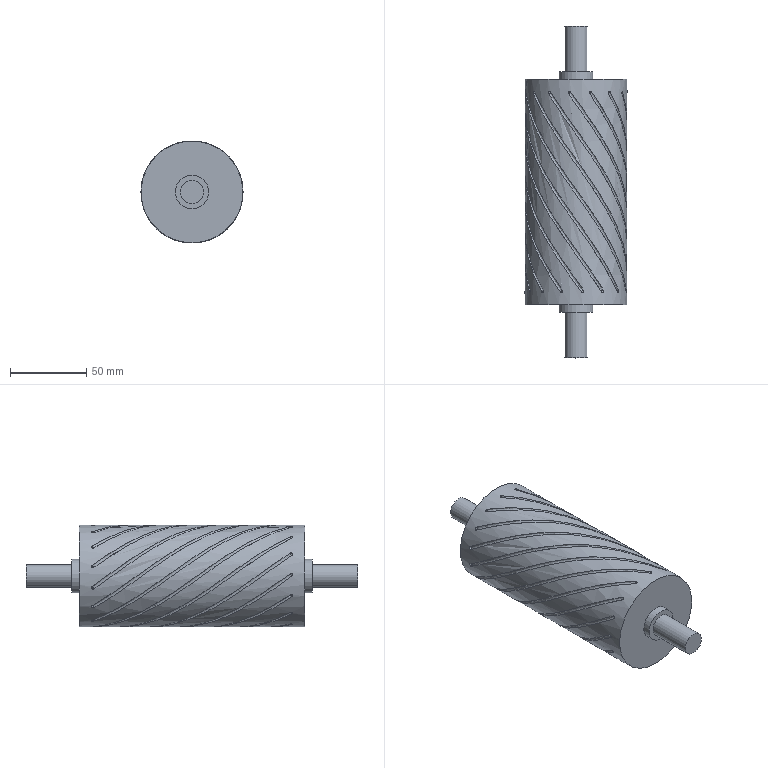Part | STEP file | YBQDJ-PD-10 | 1 solid | 86 faces | box 68.992 x 218 x 68.953 mm | volume 532441 mm3 | spline 45 | plane 36 | cylinder 5 | commonest cylinder face diameters 15 x2 22 x2 67 x1